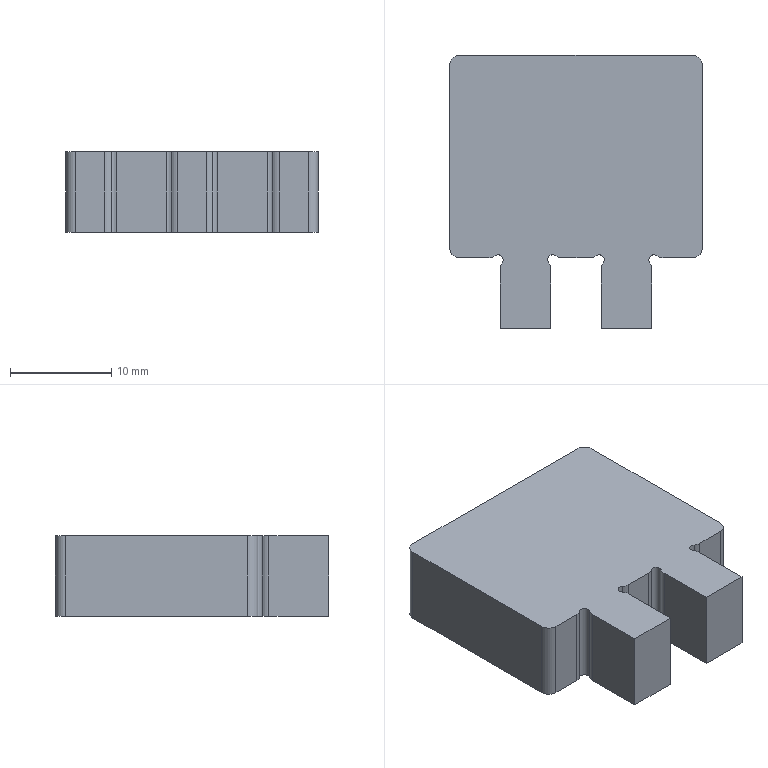Part | SolidWorks | features Fillet 1, FlatPattern 1, ICE 1, SMBaseFlange 1, SheetMetal 1 | 1 solid | 32 faces | box 25 x 27 x 8 mm | volume 4541 mm3 | cylinder 18 | plane 14 | commonest cylinder face diameters 2 x12 1 x6
STEP:
#1=CARTESIAN_POINT('',(52.732,-33.449,0.));
#2=VERTEX_POINT('',#1);
#3=CARTESIAN_POINT('',(51.932,-33.849,0.));
#4=VERTEX_POINT('',#3);
#5=CARTESIAN_POINT('',(52.432,-33.849,0.));
#6=DIRECTION('',(0.,0.,1.));
#7=DIRECTION('',(1.,0.,0.));
#8=AXIS2_PLACEMENT_3D('',#5,#6,#7);
#9=CIRCLE('',#8,0.5);
#10=EDGE_CURVE('',#2,#4,#9,.T.);
#11=ORIENTED_EDGE('',*,*,#10,.T.);
#12=CARTESIAN_POINT('',(51.932,-33.849,-8.));
#13=VERTEX_POINT('',#12);
#14=CARTESIAN_POINT('',(51.932,-33.849,-8.));
#15=DIRECTION('',(0.,0.,-1.));
#16=VECTOR('',#15,1000.);
#17=LINE('',#14,#16);
#18=EDGE_CURVE('',#4,#13,#17,.T.);
#19=ORIENTED_EDGE('',*,*,#18,.T.);
#20=CARTESIAN_POINT('',(52.732,-33.449,-8.));
#21=VERTEX_POINT('',#20);
#22=CARTESIAN_POINT('',(52.432,-33.849,-8.));
#23=DIRECTION('',(0.,0.,1.));
#24=DIRECTION('',(1.,0.,0.));
#25=AXIS2_PLACEMENT_3D('',#22,#23,#24);
#26=CIRCLE('',#25,0.5);
#27=EDGE_CURVE('',#21,#13,#26,.T.);
#28=ORIENTED_EDGE('',*,*,#27,.F.);
#29=CARTESIAN_POINT('',(52.732,-33.449,-8.));
#30=DIRECTION('',(0.,0.,1.));
#31=VECTOR('',#30,1000.);
#32=LINE('',#29,#31);
#33=EDGE_CURVE('',#21,#2,#32,.T.);
#34=ORIENTED_EDGE('',*,*,#33,.T.);
#35=EDGE_LOOP('',(#11,#19,#28,#34));
#36=FACE_OUTER_BOUND('',#35,.T.);
#37=CARTESIAN_POINT('',(52.432,-33.849,-8.));
#38=DIRECTION('',(0.,0.,-1.));
#39=DIRECTION('',(-1.,0.,0.));
#40=AXIS2_PLACEMENT_3D('',#37,#38,#39);
#41=CYLINDRICAL_SURFACE('',#40,0.5);
#42=ADVANCED_FACE('',(#36),#41,.F.);
#43=CARTESIAN_POINT('',(42.732,-33.449,0.));
#44=VERTEX_POINT('',#43);
#45=CARTESIAN_POINT('',(41.932,-33.849,0.));
#46=VERTEX_POINT('',#45);
#47=CARTESIAN_POINT('',(42.432,-33.849,0.));
#48=DIRECTION('',(0.,0.,1.));
#49=DIRECTION('',(1.,0.,0.));
#50=AXIS2_PLACEMENT_3D('',#47,#48,#49);
#51=CIRCLE('',#50,0.5);
#52=EDGE_CURVE('',#44,#46,#51,.T.);
#53=ORIENTED_EDGE('',*,*,#52,.T.);
#54=CARTESIAN_POINT('',(41.932,-33.849,-8.));
#55=VERTEX_POINT('',#54);
#56=CARTESIAN_POINT('',(41.932,-33.849,-8.));
#57=DIRECTION('',(0.,0.,-1.));
#58=VECTOR('',#57,1000.);
#59=LINE('',#56,#58);
#60=EDGE_CURVE('',#46,#55,#59,.T.);
#61=ORIENTED_EDGE('',*,*,#60,.T.);
#62=CARTESIAN_POINT('',(42.732,-33.449,-8.));
#63=VERTEX_POINT('',#62);
#64=CARTESIAN_POINT('',(42.432,-33.849,-8.));
#65=DIRECTION('',(0.,0.,1.));
#66=DIRECTION('',(1.,0.,0.));
#67=AXIS2_PLACEMENT_3D('',#64,#65,#66);
#68=CIRCLE('',#67,0.5);
#69=EDGE_CURVE('',#63,#55,#68,.T.);
#70=ORIENTED_EDGE('',*,*,#69,.F.);
#71=CARTESIAN_POINT('',(42.732,-33.449,-8.));
#72=DIRECTION('',(0.,0.,1.));
#73=VECTOR('',#72,1000.);
#74=LINE('',#71,#73);
#75=EDGE_CURVE('',#63,#44,#74,.T.);
#76=ORIENTED_EDGE('',*,*,#75,.T.);
#77=EDGE_LOOP('',(#53,#61,#70,#76));
#78=FACE_OUTER_BOUND('',#77,.T.);
#79=CARTESIAN_POINT('',(42.432,-33.849,-8.));
#80=DIRECTION('',(0.,0.,-1.));
#81=DIRECTION('',(-1.,0.,0.));
#82=AXIS2_PLACEMENT_3D('',#79,#80,#81);
#83=CYLINDRICAL_SURFACE('',#82,0.5);
#84=ADVANCED_FACE('',(#78),#83,.F.);
#85=CARTESIAN_POINT('',(33.232,-33.649,-8.));
#86=VERTEX_POINT('',#85);
#87=CARTESIAN_POINT('',(36.132,-33.649,-8.));
#88=VERTEX_POINT('',#87);
#89=CARTESIAN_POINT('',(37.232,-33.649,-8.));
#90=DIRECTION('',(1.,0.,0.));
#91=VECTOR('',#90,1000.);
#92=LINE('',#89,#91);
#93=EDGE_CURVE('',#86,#88,#92,.T.);
#94=ORIENTED_EDGE('',*,*,#93,.T.);
#95=CARTESIAN_POINT('',(36.132,-33.649,0.));
#96=VERTEX_POINT('',#95);
#97=CARTESIAN_POINT('',(36.132,-33.649,-8.));
#98=DIRECTION('',(0.,0.,1.));
#99=VECTOR('',#98,1000.);
#100=LINE('',#97,#99);
#101=EDGE_CURVE('',#88,#96,#100,.T.);
#102=ORIENTED_EDGE('',*,*,#101,.T.);
#103=CARTESIAN_POINT('',(33.232,-33.649,0.));
#104=VERTEX_POINT('',#103);
#105=CARTESIAN_POINT('',(37.232,-33.649,0.));
#106=DIRECTION('',(1.,0.,0.));
#107=VECTOR('',#106,1000.);
#108=LINE('',#105,#107);
#109=EDGE_CURVE('',#104,#96,#108,.T.);
#110=ORIENTED_EDGE('',*,*,#109,.F.);
#111=CARTESIAN_POINT('',(33.232,-33.649,-8.));
#112=DIRECTION('',(0.,0.,-1.));
#113=VECTOR('',#112,1000.);
#114=LINE('',#111,#113);
#115=EDGE_CURVE('',#104,#86,#114,.T.);
#116=ORIENTED_EDGE('',*,*,#115,.T.);
#117=EDGE_LOOP('',(#94,#102,#110,#116));
#118=FACE_OUTER_BOUND('',#117,.T.);
#119=CARTESIAN_POINT('',(37.232,-33.649,-8.));
#120=DIRECTION('',(0.,-1.,0.));
#121=DIRECTION('',(0.,0.,-1.));
#122=AXIS2_PLACEMENT_3D('',#119,#120,#121);
#123=PLANE('',#122);
#124=ADVANCED_FACE('',(#118),#123,.T.);
#125=CARTESIAN_POINT('',(53.332,-33.649,0.));
#126=VERTEX_POINT('',#125);
#127=CARTESIAN_POINT('',(56.232,-33.649,0.));
#128=VERTEX_POINT('',#127);
#129=CARTESIAN_POINT('',(57.232,-33.649,0.));
#130=DIRECTION('',(1.,0.,0.));
#131=VECTOR('',#130,1000.);
#132=LINE('',#129,#131);
#133=EDGE_CURVE('',#126,#128,#132,.T.);
#134=ORIENTED_EDGE('',*,*,#133,.F.);
#135=CARTESIAN_POINT('',(53.332,-33.649,-8.));
#136=VERTEX_POINT('',#135);
#137=CARTESIAN_POINT('',(53.332,-33.649,-8.));
#138=DIRECTION('',(0.,0.,-1.));
#139=VECTOR('',#138,1000.);
#140=LINE('',#137,#139);
#141=EDGE_CURVE('',#126,#136,#140,.T.);
#142=ORIENTED_EDGE('',*,*,#141,.T.);
#143=CARTESIAN_POINT('',(56.232,-33.649,-8.));
#144=VERTEX_POINT('',#143);
#145=CARTESIAN_POINT('',(57.232,-33.649,-8.));
#146=DIRECTION('',(1.,0.,0.));
#147=VECTOR('',#146,1000.);
#148=LINE('',#145,#147);
#149=EDGE_CURVE('',#136,#144,#148,.T.);
#150=ORIENTED_EDGE('',*,*,#149,.T.);
#151=CARTESIAN_POINT('',(56.232,-33.649,-8.));
#152=DIRECTION('',(0.,0.,1.));
#153=VECTOR('',#152,1000.);
#154=LINE('',#151,#153);
#155=EDGE_CURVE('',#144,#128,#154,.T.);
#156=ORIENTED_EDGE('',*,*,#155,.T.);
#157=EDGE_LOOP('',(#134,#142,#150,#156));
#158=FACE_OUTER_BOUND('',#157,.T.);
#159=CARTESIAN_POINT('',(57.232,-33.649,-8.));
#160=DIRECTION('',(0.,-1.,0.));
#161=DIRECTION('',(1.,0.,0.));
#162=AXIS2_PLACEMENT_3D('',#159,#160,#161);
#163=PLANE('',#162);
#164=ADVANCED_FACE('',(#158),#163,.T.);
#165=CARTESIAN_POINT('',(52.232,-40.649,-8.));
#166=VERTEX_POINT('',#165);
#167=CARTESIAN_POINT('',(52.232,-34.749,-8.));
#168=VERTEX_POINT('',#167);
#169=CARTESIAN_POINT('',(52.232,-33.649,-8.));
#170=DIRECTION('',(0.,1.,0.));
#171=VECTOR('',#170,1000.);
#172=LINE('',#169,#171);
#173=EDGE_CURVE('',#166,#168,#172,.T.);
#174=ORIENTED_EDGE('',*,*,#173,.T.);
#175=CARTESIAN_POINT('',(52.232,-34.749,0.));
#176=VERTEX_POINT('',#175);
#177=CARTESIAN_POINT('',(52.232,-34.749,-8.));
#178=DIRECTION('',(0.,0.,1.));
#179=VECTOR('',#178,1000.);
#180=LINE('',#177,#179);
#181=EDGE_CURVE('',#168,#176,#180,.T.);
#182=ORIENTED_EDGE('',*,*,#181,.T.);
#183=CARTESIAN_POINT('',(52.232,-40.649,0.));
#184=VERTEX_POINT('',#183);
#185=CARTESIAN_POINT('',(52.232,-33.649,0.));
#186=DIRECTION('',(0.,1.,0.));
#187=VECTOR('',#186,1000.);
#188=LINE('',#185,#187);
#189=EDGE_CURVE('',#184,#176,#188,.T.);
#190=ORIENTED_EDGE('',*,*,#189,.F.);
#191=CARTESIAN_POINT('',(52.232,-40.649,-8.));
#192=DIRECTION('',(0.,0.,1.));
#193=VECTOR('',#192,1000.);
#194=LINE('',#191,#193);
#195=EDGE_CURVE('',#166,#184,#194,.T.);
#196=ORIENTED_EDGE('',*,*,#195,.F.);
#197=EDGE_LOOP('',(#174,#182,#190,#196));
#198=FACE_OUTER_BOUND('',#197,.T.);
#199=CARTESIAN_POINT('',(52.232,-33.649,-8.));
#200=DIRECTION('',(1.,0.,0.));
#201=DIRECTION('',(0.,0.,-1.));
#202=AXIS2_PLACEMENT_3D('',#199,#200,#201);
#203=PLANE('',#202);
#204=ADVANCED_FACE('',(#198),#203,.T.);
#205=CARTESIAN_POINT('',(47.232,-34.749,0.));
#206=VERTEX_POINT('',#205);
#207=CARTESIAN_POINT('',(47.232,-40.649,0.));
#208=VERTEX_POINT('',#207);
#209=CARTESIAN_POINT('',(47.232,-40.649,0.));
#210=DIRECTION('',(0.,-1.,0.));
#211=VECTOR('',#210,1000.);
#212=LINE('',#209,#211);
#213=EDGE_CURVE('',#206,#208,#212,.T.);
#214=ORIENTED_EDGE('',*,*,#213,.F.);
#215=CARTESIAN_POINT('',(47.232,-34.749,-8.));
#216=VERTEX_POINT('',#215);
#217=CARTESIAN_POINT('',(47.232,-34.749,-8.));
#218=DIRECTION('',(0.,0.,-1.));
#219=VECTOR('',#218,1000.);
#220=LINE('',#217,#219);
#221=EDGE_CURVE('',#206,#216,#220,.T.);
#222=ORIENTED_EDGE('',*,*,#221,.T.);
#223=CARTESIAN_POINT('',(47.232,-40.649,-8.));
#224=VERTEX_POINT('',#223);
#225=CARTESIAN_POINT('',(47.232,-40.649,-8.));
#226=DIRECTION('',(0.,-1.,0.));
#227=VECTOR('',#226,1000.);
#228=LINE('',#225,#227);
#229=EDGE_CURVE('',#216,#224,#228,.T.);
#230=ORIENTED_EDGE('',*,*,#229,.T.);
#231=CARTESIAN_POINT('',(47.232,-40.649,-8.));
#232=DIRECTION('',(0.,0.,1.));
#233=VECTOR('',#232,1000.);
#234=LINE('',#231,#233);
#235=EDGE_CURVE('',#224,#208,#234,.T.);
#236=ORIENTED_EDGE('',*,*,#235,.T.);
#237=EDGE_LOOP('',(#214,#222,#230,#236));
#238=FACE_OUTER_BOUND('',#237,.T.);
#239=CARTESIAN_POINT('',(47.232,-40.649,-8.));
#240=DIRECTION('',(-1.,0.,0.));
#241=DIRECTION('',(0.,0.,1.));
#242=AXIS2_PLACEMENT_3D('',#239,#240,#241);
#243=PLANE('',#242);
#244=ADVANCED_FACE('',(#238),#243,.T.);
#245=CARTESIAN_POINT('',(43.332,-33.649,-8.));
#246=VERTEX_POINT('',#245);
#247=CARTESIAN_POINT('',(46.132,-33.649,-8.));
#248=VERTEX_POINT('',#247);
#249=CARTESIAN_POINT('',(47.232,-33.649,-8.));
#250=DIRECTION('',(1.,0.,0.));
#251=VECTOR('',#250,1000.);
#252=LINE('',#249,#251);
#253=EDGE_CURVE('',#246,#248,#252,.T.);
#254=ORIENTED_EDGE('',*,*,#253,.T.);
#255=CARTESIAN_POINT('',(46.132,-33.649,0.));
#256=VERTEX_POINT('',#255);
#257=CARTESIAN_POINT('',(46.132,-33.649,-8.));
#258=DIRECTION('',(0.,0.,1.));
#259=VECTOR('',#258,1000.);
#260=LINE('',#257,#259);
#261=EDGE_CURVE('',#248,#256,#260,.T.);
#262=ORIENTED_EDGE('',*,*,#261,.T.);
#263=CARTESIAN_POINT('',(43.332,-33.649,0.));
#264=VERTEX_POINT('',#263);
#265=CARTESIAN_POINT('',(47.232,-33.649,0.));
#266=DIRECTION('',(1.,0.,0.));
#267=VECTOR('',#266,1000.);
#268=LINE('',#265,#267);
#269=EDGE_CURVE('',#264,#256,#268,.T.);
#270=ORIENTED_EDGE('',*,*,#269,.F.);
#271=CARTESIAN_POINT('',(43.332,-33.649,-8.));
#272=DIRECTION('',(0.,0.,-1.));
#273=VECTOR('',#272,1000.);
#274=LINE('',#271,#273);
#275=EDGE_CURVE('',#264,#246,#274,.T.);
#276=ORIENTED_EDGE('',*,*,#275,.T.);
#277=EDGE_LOOP('',(#254,#262,#270,#276));
#278=FACE_OUTER_BOUND('',#277,.T.);
#279=CARTESIAN_POINT('',(47.232,-33.649,-8.));
#280=DIRECTION('',(0.,-1.,0.));
#281=DIRECTION('',(1.,0.,0.));
#282=AXIS2_PLACEMENT_3D('',#279,#280,#281);
#283=PLANE('',#282);
#284=ADVANCED_FACE('',(#278),#283,.T.);
#285=CARTESIAN_POINT('',(42.232,-40.649,-8.));
#286=VERTEX_POINT('',#285);
#287=CARTESIAN_POINT('',(42.232,-34.749,-8.));
#288=VERTEX_POINT('',#287);
#289=CARTESIAN_POINT('',(42.232,-33.649,-8.));
#290=DIRECTION('',(0.,1.,0.));
#291=VECTOR('',#290,1000.);
#292=LINE('',#289,#291);
#293=EDGE_CURVE('',#286,#288,#292,.T.);
#294=ORIENTED_EDGE('',*,*,#293,.T.);
#295=CARTESIAN_POINT('',(42.232,-34.749,0.));
#296=VERTEX_POINT('',#295);
#297=CARTESIAN_POINT('',(42.232,-34.749,-8.));
#298=DIRECTION('',(0.,0.,1.));
#299=VECTOR('',#298,1000.);
#300=LINE('',#297,#299);
#301=EDGE_CURVE('',#288,#296,#300,.T.);
#302=ORIENTED_EDGE('',*,*,#301,.T.);
#303=CARTESIAN_POINT('',(42.232,-40.649,0.));
#304=VERTEX_POINT('',#303);
#305=CARTESIAN_POINT('',(42.232,-33.649,0.));
#306=DIRECTION('',(0.,1.,0.));
#307=VECTOR('',#306,1000.);
#308=LINE('',#305,#307);
#309=EDGE_CURVE('',#304,#296,#308,.T.);
#310=ORIENTED_EDGE('',*,*,#309,.F.);
#311=CARTESIAN_POINT('',(42.232,-40.649,-8.));
#312=DIRECTION('',(0.,0.,1.));
#313=VECTOR('',#312,1000.);
#314=LINE('',#311,#313);
#315=EDGE_CURVE('',#286,#304,#314,.T.);
#316=ORIENTED_EDGE('',*,*,#315,.F.);
#317=EDGE_LOOP('',(#294,#302,#310,#316));
#318=FACE_OUTER_BOUND('',#317,.T.);
#319=CARTESIAN_POINT('',(42.232,-33.649,-8.));
#320=DIRECTION('',(1.,0.,0.));
#321=DIRECTION('',(0.,0.,-1.));
#322=AXIS2_PLACEMENT_3D('',#319,#320,#321);
#323=PLANE('',#322);
#324=ADVANCED_FACE('',(#318),#323,.T.);
#325=CARTESIAN_POINT('',(37.232,-34.749,0.));
#326=VERTEX_POINT('',#325);
#327=CARTESIAN_POINT('',(37.232,-40.649,0.));
#328=VERTEX_POINT('',#327);
#329=CARTESIAN_POINT('',(37.232,-40.649,0.));
#330=DIRECTION('',(0.,-1.,0.));
#331=VECTOR('',#330,1000.);
#332=LINE('',#329,#331);
#333=EDGE_CURVE('',#326,#328,#332,.T.);
#334=ORIENTED_EDGE('',*,*,#333,.F.);
#335=CARTESIAN_POINT('',(37.232,-34.749,-8.));
#336=VERTEX_POINT('',#335);
#337=CARTESIAN_POINT('',(37.232,-34.749,-8.));
#338=DIRECTION('',(0.,0.,-1.));
#339=VECTOR('',#338,1000.);
#340=LINE('',#337,#339);
#341=EDGE_CURVE('',#326,#336,#340,.T.);
#342=ORIENTED_EDGE('',*,*,#341,.T.);
#343=CARTESIAN_POINT('',(37.232,-40.649,-8.));
#344=VERTEX_POINT('',#343);
#345=CARTESIAN_POINT('',(37.232,-40.649,-8.));
#346=DIRECTION('',(0.,-1.,0.));
#347=VECTOR('',#346,1000.);
#348=LINE('',#345,#347);
#349=EDGE_CURVE('',#336,#344,#348,.T.);
#350=ORIENTED_EDGE('',*,*,#349,.T.);
#351=CARTESIAN_POINT('',(37.232,-40.649,-8.));
#352=DIRECTION('',(0.,0.,1.));
#353=VECTOR('',#352,1000.);
#354=LINE('',#351,#353);
#355=EDGE_CURVE('',#344,#328,#354,.T.);
#356=ORIENTED_EDGE('',*,*,#355,.T.);
#357=EDGE_LOOP('',(#334,#342,#350,#356));
#358=FACE_OUTER_BOUND('',#357,.T.);
#359=CARTESIAN_POINT('',(37.232,-40.649,-8.));
#360=DIRECTION('',(-1.,0.,0.));
#361=DIRECTION('',(0.,0.,1.));
#362=AXIS2_PLACEMENT_3D('',#359,#360,#361);
#363=PLANE('',#362);
#364=ADVANCED_FACE('',(#358),#363,.T.);
#365=CARTESIAN_POINT('',(32.232,-14.649,-8.));
#366=VERTEX_POINT('',#365);
#367=CARTESIAN_POINT('',(32.232,-32.649,-8.));
#368=VERTEX_POINT('',#367);
#369=CARTESIAN_POINT('',(32.232,-33.649,-8.));
#370=DIRECTION('',(0.,-1.,0.));
#371=VECTOR('',#370,1000.);
#372=LINE('',#369,#371);
#373=EDGE_CURVE('',#366,#368,#372,.T.);
#374=ORIENTED_EDGE('',*,*,#373,.T.);
#375=CARTESIAN_POINT('',(32.232,-32.649,0.));
#376=VERTEX_POINT('',#375);
#377=CARTESIAN_POINT('',(32.232,-32.649,-8.));
#378=DIRECTION('',(0.,0.,1.));
#379=VECTOR('',#378,1000.);
#380=LINE('',#377,#379);
#381=EDGE_CURVE('',#368,#376,#380,.T.);
#382=ORIENTED_EDGE('',*,*,#381,.T.);
#383=CARTESIAN_POINT('',(32.232,-14.649,0.));
#384=VERTEX_POINT('',#383);
#385=CARTESIAN_POINT('',(32.232,-33.649,0.));
#386=DIRECTION('',(0.,-1.,0.));
#387=VECTOR('',#386,1000.);
#388=LINE('',#385,#387);
#389=EDGE_CURVE('',#384,#376,#388,.T.);
#390=ORIENTED_EDGE('',*,*,#389,.F.);
#391=CARTESIAN_POINT('',(32.232,-14.649,-8.));
#392=DIRECTION('',(0.,0.,-1.));
#393=VECTOR('',#392,1000.);
#394=LINE('',#391,#393);
#395=EDGE_CURVE('',#384,#366,#394,.T.);
#396=ORIENTED_EDGE('',*,*,#395,.T.);
#397=EDGE_LOOP('',(#374,#382,#390,#396));
#398=FACE_OUTER_BOUND('',#397,.T.);
#399=CARTESIAN_POINT('',(32.232,-33.649,-8.));
#400=DIRECTION('',(-1.,0.,0.));
#401=DIRECTION('',(0.,0.,1.));
#402=AXIS2_PLACEMENT_3D('',#399,#400,#401);
#403=PLANE('',#402);
#404=ADVANCED_FACE('',(#398),#403,.T.);
#405=CARTESIAN_POINT('',(56.232,-13.649,-8.));
#406=VERTEX_POINT('',#405);
#407=CARTESIAN_POINT('',(33.232,-13.649,-8.));
#408=VERTEX_POINT('',#407);
#409=CARTESIAN_POINT('',(32.232,-13.649,-8.));
#410=DIRECTION('',(-1.,0.,0.));
#411=VECTOR('',#410,1000.);
#412=LINE('',#409,#411);
#413=EDGE_CURVE('',#406,#408,#412,.T.);
#414=ORIENTED_EDGE('',*,*,#413,.T.);
#415=CARTESIAN_POINT('',(33.232,-13.649,0.));
#416=VERTEX_POINT('',#415);
#417=CARTESIAN_POINT('',(33.232,-13.649,-8.));
#418=DIRECTION('',(0.,0.,1.));
#419=VECTOR('',#418,1000.);
#420=LINE('',#417,#419);
#421=EDGE_CURVE('',#408,#416,#420,.T.);
#422=ORIENTED_EDGE('',*,*,#421,.T.);
#423=CARTESIAN_POINT('',(56.232,-13.649,0.));
#424=VERTEX_POINT('',#423);
#425=CARTESIAN_POINT('',(32.232,-13.649,0.));
#426=DIRECTION('',(-1.,0.,0.));
#427=VECTOR('',#426,1000.);
#428=LINE('',#425,#427);
#429=EDGE_CURVE('',#424,#416,#428,.T.);
#430=ORIENTED_EDGE('',*,*,#429,.F.);
#431=CARTESIAN_POINT('',(56.232,-13.649,-8.));
#432=DIRECTION('',(0.,0.,-1.));
#433=VECTOR('',#432,1000.);
#434=LINE('',#431,#433);
#435=EDGE_CURVE('',#424,#406,#434,.T.);
#436=ORIENTED_EDGE('',*,*,#435,.T.);
#437=EDGE_LOOP('',(#414,#422,#430,#436));
#438=FACE_OUTER_BOUND('',#437,.T.);
#439=CARTESIAN_POINT('',(32.232,-13.649,-8.));
#440=DIRECTION('',(0.,1.,0.));
#441=DIRECTION('',(0.,0.,1.));
#442=AXIS2_PLACEMENT_3D('',#439,#440,#441);
#443=PLANE('',#442);
#444=ADVANCED_FACE('',(#438),#443,.T.);
#445=CARTESIAN_POINT('',(57.232,-32.649,0.));
#446=VERTEX_POINT('',#445);
#447=CARTESIAN_POINT('',(57.232,-14.649,0.));
#448=VERTEX_POINT('',#447);
#449=CARTESIAN_POINT('',(57.232,-13.649,0.));
#450=DIRECTION('',(0.,1.,0.));
#451=VECTOR('',#450,1000.);
#452=LINE('',#449,#451);
#453=EDGE_CURVE('',#446,#448,#452,.T.);
#454=ORIENTED_EDGE('',*,*,#453,.F.);
#455=CARTESIAN_POINT('',(57.232,-32.649,-8.));
#456=VERTEX_POINT('',#455);
#457=CARTESIAN_POINT('',(57.232,-32.649,-8.));
#458=DIRECTION('',(0.,0.,-1.));
#459=VECTOR('',#458,1000.);
#460=LINE('',#457,#459);
#461=EDGE_CURVE('',#446,#456,#460,.T.);
#462=ORIENTED_EDGE('',*,*,#461,.T.);
#463=CARTESIAN_POINT('',(57.232,-14.649,-8.));
#464=VERTEX_POINT('',#463);
#465=CARTESIAN_POINT('',(57.232,-13.649,-8.));
#466=DIRECTION('',(0.,1.,0.));
#467=VECTOR('',#466,1000.);
#468=LINE('',#465,#467);
#469=EDGE_CURVE('',#456,#464,#468,.T.);
#470=ORIENTED_EDGE('',*,*,#469,.T.);
#471=CARTESIAN_POINT('',(57.232,-14.649,-8.));
#472=DIRECTION('',(0.,0.,1.));
#473=VECTOR('',#472,1000.);
#474=LINE('',#471,#473);
#475=EDGE_CURVE('',#464,#448,#474,.T.);
#476=ORIENTED_EDGE('',*,*,#475,.T.);
#477=EDGE_LOOP('',(#454,#462,#470,#476));
#478=FACE_OUTER_BOUND('',#477,.T.);
#479=CARTESIAN_POINT('',(57.232,-13.649,-8.));
#480=DIRECTION('',(1.,0.,0.));
#481=DIRECTION('',(0.,0.,-1.));
#482=AXIS2_PLACEMENT_3D('',#479,#480,#481);
#483=PLANE('',#482);
#484=ADVANCED_FACE('',(#478),#483,.T.);
#485=CARTESIAN_POINT('',(52.232,-40.649,0.));
#486=DIRECTION('',(1.,0.,0.));
#487=VECTOR('',#486,1000.);
#488=LINE('',#485,#487);
#489=EDGE_CURVE('',#208,#184,#488,.T.);
#490=ORIENTED_EDGE('',*,*,#489,.F.);
#491=ORIENTED_EDGE('',*,*,#235,.F.);
#492=CARTESIAN_POINT('',(52.232,-40.649,-8.));
#493=DIRECTION('',(1.,0.,0.));
#494=VECTOR('',#493,1000.);
#495=LINE('',#492,#494);
#496=EDGE_CURVE('',#224,#166,#495,.T.);
#497=ORIENTED_EDGE('',*,*,#496,.T.);
#498=ORIENTED_EDGE('',*,*,#195,.T.);
#499=EDGE_LOOP('',(#490,#491,#497,#498));
#500=FACE_OUTER_BOUND('',#499,.T.);
#501=CARTESIAN_POINT('',(52.232,-40.649,-8.));
#502=DIRECTION('',(0.,-1.,0.));
#503=DIRECTION('',(1.,0.,0.));
#504=AXIS2_PLACEMENT_3D('',#501,#502,#503);
#505=PLANE('',#504);
#506=ADVANCED_FACE('',(#500),#505,.T.);
#507=CARTESIAN_POINT('',(42.232,-40.649,0.));
#508=DIRECTION('',(1.,0.,0.));
#509=VECTOR('',#508,1000.);
#510=LINE('',#507,#509);
#511=EDGE_CURVE('',#328,#304,#510,.T.);
#512=ORIENTED_EDGE('',*,*,#511,.F.);
#513=ORIENTED_EDGE('',*,*,#355,.F.);
#514=CARTESIAN_POINT('',(42.232,-40.649,-8.));
#515=DIRECTION('',(1.,0.,0.));
#516=VECTOR('',#515,1000.);
#517=LINE('',#514,#516);
#518=EDGE_CURVE('',#344,#286,#517,.T.);
#519=ORIENTED_EDGE('',*,*,#518,.T.);
#520=ORIENTED_EDGE('',*,*,#315,.T.);
#521=EDGE_LOOP('',(#512,#513,#519,#520));
#522=FACE_OUTER_BOUND('',#521,.T.);
#523=CARTESIAN_POINT('',(42.232,-40.649,-8.));
#524=DIRECTION('',(0.,-1.,0.));
#525=DIRECTION('',(0.,0.,-1.));
#526=AXIS2_PLACEMENT_3D('',#523,#524,#525);
#527=PLANE('',#526);
#528=ADVANCED_FACE('',(#522),#527,.T.);
#529=ORIENTED_EDGE('',*,*,#149,.F.);
#530=CARTESIAN_POINT('',(53.332,-32.649,-8.));
#531=DIRECTION('',(0.,0.,-1.));
#532=DIRECTION('',(-1.,0.,0.));
#533=AXIS2_PLACEMENT_3D('',#530,#531,#532);
#534=CIRCLE('',#533,1.);
#535=EDGE_CURVE('',#136,#21,#534,.T.);
#536=ORIENTED_EDGE('',*,*,#535,.T.);
#537=ORIENTED_EDGE('',*,*,#27,.T.);
#538=CARTESIAN_POINT('',(52.032,-34.149,-8.));
#539=VERTEX_POINT('',#538);
#540=CARTESIAN_POINT('',(52.432,-33.849,-8.));
#541=DIRECTION('',(0.,0.,1.));
#542=DIRECTION('',(1.,0.,0.));
#543=AXIS2_PLACEMENT_3D('',#540,#541,#542);
#544=CIRCLE('',#543,0.5);
#545=EDGE_CURVE('',#13,#539,#544,.T.);
#546=ORIENTED_EDGE('',*,*,#545,.T.);
#547=CARTESIAN_POINT('',(51.232,-34.749,-8.));
#548=DIRECTION('',(0.,0.,-1.));
#549=DIRECTION('',(-1.,0.,0.));
#550=AXIS2_PLACEMENT_3D('',#547,#548,#549);
#551=CIRCLE('',#550,1.);
#552=EDGE_CURVE('',#539,#168,#551,.T.);
#553=ORIENTED_EDGE('',*,*,#552,.T.);
#554=ORIENTED_EDGE('',*,*,#173,.F.);
#555=ORIENTED_EDGE('',*,*,#496,.F.);
#556=ORIENTED_EDGE('',*,*,#229,.F.);
#557=CARTESIAN_POINT('',(47.432,-34.149,-8.));
#558=VERTEX_POINT('',#557);
#559=CARTESIAN_POINT('',(48.232,-34.749,-8.));
#560=DIRECTION('',(0.,0.,-1.));
#561=DIRECTION('',(-1.,0.,0.));
#562=AXIS2_PLACEMENT_3D('',#559,#560,#561);
#563=CIRCLE('',#562,1.);
#564=EDGE_CURVE('',#216,#558,#563,.T.);
#565=ORIENTED_EDGE('',*,*,#564,.T.);
#566=CARTESIAN_POINT('',(46.732,-33.449,-8.));
#567=VERTEX_POINT('',#566);
#568=CARTESIAN_POINT('',(47.032,-33.849,-8.));
#569=DIRECTION('',(0.,0.,1.));
#570=DIRECTION('',(1.,0.,0.));
#571=AXIS2_PLACEMENT_3D('',#568,#569,#570);
#572=CIRCLE('',#571,0.5);
#573=EDGE_CURVE('',#558,#567,#572,.T.);
#574=ORIENTED_EDGE('',*,*,#573,.T.);
#575=CARTESIAN_POINT('',(46.132,-32.649,-8.));
#576=DIRECTION('',(0.,0.,-1.));
#577=DIRECTION('',(-1.,0.,0.));
#578=AXIS2_PLACEMENT_3D('',#575,#576,#577);
#579=CIRCLE('',#578,1.);
#580=EDGE_CURVE('',#567,#248,#579,.T.);
#581=ORIENTED_EDGE('',*,*,#580,.T.);
#582=ORIENTED_EDGE('',*,*,#253,.F.);
#583=CARTESIAN_POINT('',(43.332,-32.649,-8.));
#584=DIRECTION('',(0.,0.,-1.));
#585=DIRECTION('',(-1.,0.,0.));
#586=AXIS2_PLACEMENT_3D('',#583,#584,#585);
#587=CIRCLE('',#586,1.);
#588=EDGE_CURVE('',#246,#63,#587,.T.);
#589=ORIENTED_EDGE('',*,*,#588,.T.);
#590=ORIENTED_EDGE('',*,*,#69,.T.);
#591=CARTESIAN_POINT('',(42.032,-34.149,-8.));
#592=VERTEX_POINT('',#591);
#593=CARTESIAN_POINT('',(42.432,-33.849,-8.));
#594=DIRECTION('',(0.,0.,1.));
#595=DIRECTION('',(1.,0.,0.));
#596=AXIS2_PLACEMENT_3D('',#593,#594,#595);
#597=CIRCLE('',#596,0.5);
#598=EDGE_CURVE('',#55,#592,#597,.T.);
#599=ORIENTED_EDGE('',*,*,#598,.T.);
#600=CARTESIAN_POINT('',(41.232,-34.749,-8.));
#601=DIRECTION('',(0.,0.,-1.));
#602=DIRECTION('',(-1.,0.,0.));
#603=AXIS2_PLACEMENT_3D('',#600,#601,#602);
#604=CIRCLE('',#603,1.);
#605=EDGE_CURVE('',#592,#288,#604,.T.);
#606=ORIENTED_EDGE('',*,*,#605,.T.);
#607=ORIENTED_EDGE('',*,*,#293,.F.);
#608=ORIENTED_EDGE('',*,*,#518,.F.);
#609=ORIENTED_EDGE('',*,*,#349,.F.);
#610=CARTESIAN_POINT('',(37.432,-34.149,-8.));
#611=VERTEX_POINT('',#610);
#612=CARTESIAN_POINT('',(38.232,-34.749,-8.));
#613=DIRECTION('',(0.,0.,-1.));
#614=DIRECTION('',(-1.,0.,0.));
#615=AXIS2_PLACEMENT_3D('',#612,#613,#614);
#616=CIRCLE('',#615,1.);
#617=EDGE_CURVE('',#336,#611,#616,.T.);
#618=ORIENTED_EDGE('',*,*,#617,.T.);
#619=CARTESIAN_POINT('',(36.732,-33.449,-8.));
#620=VERTEX_POINT('',#619);
#621=CARTESIAN_POINT('',(37.032,-33.849,-8.));
#622=DIRECTION('',(0.,0.,-1.));
#623=DIRECTION('',(-1.,0.,0.));
#624=AXIS2_PLACEMENT_3D('',#621,#622,#623);
#625=CIRCLE('',#624,0.5);
#626=EDGE_CURVE('',#620,#611,#625,.T.);
#627=ORIENTED_EDGE('',*,*,#626,.F.);
#628=CARTESIAN_POINT('',(36.132,-32.649,-8.));
#629=DIRECTION('',(0.,0.,-1.));
#630=DIRECTION('',(-1.,0.,0.));
#631=AXIS2_PLACEMENT_3D('',#628,#629,#630);
#632=CIRCLE('',#631,1.);
#633=EDGE_CURVE('',#620,#88,#632,.T.);
#634=ORIENTED_EDGE('',*,*,#633,.T.);
#635=ORIENTED_EDGE('',*,*,#93,.F.);
#636=CARTESIAN_POINT('',(33.232,-32.649,-8.));
#637=DIRECTION('',(0.,0.,-1.));
#638=DIRECTION('',(-1.,0.,0.));
#639=AXIS2_PLACEMENT_3D('',#636,#637,#638);
#640=CIRCLE('',#639,1.);
#641=EDGE_CURVE('',#86,#368,#640,.T.);
#642=ORIENTED_EDGE('',*,*,#641,.T.);
#643=ORIENTED_EDGE('',*,*,#373,.F.);
#644=CARTESIAN_POINT('',(33.232,-14.649,-8.));
#645=DIRECTION('',(0.,0.,-1.));
#646=DIRECTION('',(-1.,0.,0.));
#647=AXIS2_PLACEMENT_3D('',#644,#645,#646);
#648=CIRCLE('',#647,1.);
#649=EDGE_CURVE('',#366,#408,#648,.T.);
#650=ORIENTED_EDGE('',*,*,#649,.T.);
#651=ORIENTED_EDGE('',*,*,#413,.F.);
#652=CARTESIAN_POINT('',(56.232,-14.649,-8.));
#653=DIRECTION('',(0.,0.,-1.));
#654=DIRECTION('',(-1.,0.,0.));
#655=AXIS2_PLACEMENT_3D('',#652,#653,#654);
#656=CIRCLE('',#655,1.);
#657=EDGE_CURVE('',#406,#464,#656,.T.);
#658=ORIENTED_EDGE('',*,*,#657,.T.);
#659=ORIENTED_EDGE('',*,*,#469,.F.);
#660=CARTESIAN_POINT('',(56.232,-32.649,-8.));
#661=DIRECTION('',(0.,0.,-1.));
#662=DIRECTION('',(-1.,0.,0.));
#663=AXIS2_PLACEMENT_3D('',#660,#661,#662);
#664=CIRCLE('',#663,1.);
#665=EDGE_CURVE('',#456,#144,#664,.T.);
#666=ORIENTED_EDGE('',*,*,#665,.T.);
#667=EDGE_LOOP('',(#529,#536,#537,#546,#553,#554,#555,#556,#565,#574,#581,#582,#589,#590,#599,#606,#607,#608,#609,#618,#627,#634,#635,#642,#643,#650,#651,#658,#659,#666));
#668=FACE_OUTER_BOUND('',#667,.T.);
#669=CARTESIAN_POINT('',(0.,0.,-8.));
#670=DIRECTION('',(0.,0.,-1.));
#671=DIRECTION('',(-1.,0.,0.));
#672=AXIS2_PLACEMENT_3D('',#669,#670,#671);
#673=PLANE('',#672);
#674=ADVANCED_FACE('',(#668),#673,.T.);
#675=ORIENTED_EDGE('',*,*,#10,.F.);
#676=CARTESIAN_POINT('',(53.332,-32.649,0.));
#677=DIRECTION('',(0.,0.,1.));
#678=DIRECTION('',(-1.,0.,0.));
#679=AXIS2_PLACEMENT_3D('',#676,#677,#678);
#680=CIRCLE('',#679,1.);
#681=EDGE_CURVE('',#2,#126,#680,.T.);
#682=ORIENTED_EDGE('',*,*,#681,.T.);
#683=ORIENTED_EDGE('',*,*,#133,.T.);
#684=CARTESIAN_POINT('',(56.232,-32.649,0.));
#685=DIRECTION('',(0.,0.,1.));
#686=DIRECTION('',(-1.,0.,0.));
#687=AXIS2_PLACEMENT_3D('',#684,#685,#686);
#688=CIRCLE('',#687,1.);
#689=EDGE_CURVE('',#128,#446,#688,.T.);
#690=ORIENTED_EDGE('',*,*,#689,.T.);
#691=ORIENTED_EDGE('',*,*,#453,.T.);
#692=CARTESIAN_POINT('',(56.232,-14.649,0.));
#693=DIRECTION('',(0.,0.,1.));
#694=DIRECTION('',(-1.,0.,0.));
#695=AXIS2_PLACEMENT_3D('',#692,#693,#694);
#696=CIRCLE('',#695,1.);
#697=EDGE_CURVE('',#448,#424,#696,.T.);
#698=ORIENTED_EDGE('',*,*,#697,.T.);
#699=ORIENTED_EDGE('',*,*,#429,.T.);
#700=CARTESIAN_POINT('',(33.232,-14.649,0.));
#701=DIRECTION('',(0.,0.,1.));
#702=DIRECTION('',(-1.,0.,0.));
#703=AXIS2_PLACEMENT_3D('',#700,#701,#702);
#704=CIRCLE('',#703,1.);
#705=EDGE_CURVE('',#416,#384,#704,.T.);
#706=ORIENTED_EDGE('',*,*,#705,.T.);
#707=ORIENTED_EDGE('',*,*,#389,.T.);
#708=CARTESIAN_POINT('',(33.232,-32.649,0.));
#709=DIRECTION('',(0.,0.,1.));
#710=DIRECTION('',(-1.,0.,0.));
#711=AXIS2_PLACEMENT_3D('',#708,#709,#710);
#712=CIRCLE('',#711,1.);
#713=EDGE_CURVE('',#376,#104,#712,.T.);
#714=ORIENTED_EDGE('',*,*,#713,.T.);
#715=ORIENTED_EDGE('',*,*,#109,.T.);
#716=CARTESIAN_POINT('',(36.732,-33.449,0.));
#717=VERTEX_POINT('',#716);
#718=CARTESIAN_POINT('',(36.132,-32.649,0.));
#719=DIRECTION('',(0.,0.,1.));
#720=DIRECTION('',(-1.,0.,0.));
#721=AXIS2_PLACEMENT_3D('',#718,#719,#720);
#722=CIRCLE('',#721,1.);
#723=EDGE_CURVE('',#96,#717,#722,.T.);
#724=ORIENTED_EDGE('',*,*,#723,.T.);
#725=CARTESIAN_POINT('',(37.432,-34.149,0.));
#726=VERTEX_POINT('',#725);
#727=CARTESIAN_POINT('',(37.032,-33.849,0.));
#728=DIRECTION('',(0.,0.,-1.));
#729=DIRECTION('',(-1.,0.,0.));
#730=AXIS2_PLACEMENT_3D('',#727,#728,#729);
#731=CIRCLE('',#730,0.5);
#732=EDGE_CURVE('',#717,#726,#731,.T.);
#733=ORIENTED_EDGE('',*,*,#732,.T.);
#734=CARTESIAN_POINT('',(38.232,-34.749,0.));
#735=DIRECTION('',(0.,0.,1.));
#736=DIRECTION('',(-1.,0.,0.));
#737=AXIS2_PLACEMENT_3D('',#734,#735,#736);
#738=CIRCLE('',#737,1.);
#739=EDGE_CURVE('',#726,#326,#738,.T.);
#740=ORIENTED_EDGE('',*,*,#739,.T.);
#741=ORIENTED_EDGE('',*,*,#333,.T.);
#742=ORIENTED_EDGE('',*,*,#511,.T.);
#743=ORIENTED_EDGE('',*,*,#309,.T.);
#744=CARTESIAN_POINT('',(42.032,-34.149,0.));
#745=VERTEX_POINT('',#744);
#746=CARTESIAN_POINT('',(41.232,-34.749,0.));
#747=DIRECTION('',(0.,0.,1.));
#748=DIRECTION('',(-1.,0.,0.));
#749=AXIS2_PLACEMENT_3D('',#746,#747,#748);
#750=CIRCLE('',#749,1.);
#751=EDGE_CURVE('',#296,#745,#750,.T.);
#752=ORIENTED_EDGE('',*,*,#751,.T.);
#753=CARTESIAN_POINT('',(42.432,-33.849,0.));
#754=DIRECTION('',(0.,0.,1.));
#755=DIRECTION('',(1.,0.,0.));
#756=AXIS2_PLACEMENT_3D('',#753,#754,#755);
#757=CIRCLE('',#756,0.5);
#758=EDGE_CURVE('',#46,#745,#757,.T.);
#759=ORIENTED_EDGE('',*,*,#758,.F.);
#760=ORIENTED_EDGE('',*,*,#52,.F.);
#761=CARTESIAN_POINT('',(43.332,-32.649,0.));
#762=DIRECTION('',(0.,0.,1.));
#763=DIRECTION('',(-1.,0.,0.));
#764=AXIS2_PLACEMENT_3D('',#761,#762,#763);
#765=CIRCLE('',#764,1.);
#766=EDGE_CURVE('',#44,#264,#765,.T.);
#767=ORIENTED_EDGE('',*,*,#766,.T.);
#768=ORIENTED_EDGE('',*,*,#269,.T.);
#769=CARTESIAN_POINT('',(46.732,-33.449,0.));
#770=VERTEX_POINT('',#769);
#771=CARTESIAN_POINT('',(46.132,-32.649,0.));
#772=DIRECTION('',(0.,0.,1.));
#773=DIRECTION('',(-1.,0.,0.));
#774=AXIS2_PLACEMENT_3D('',#771,#772,#773);
#775=CIRCLE('',#774,1.);
#776=EDGE_CURVE('',#256,#770,#775,.T.);
#777=ORIENTED_EDGE('',*,*,#776,.T.);
#778=CARTESIAN_POINT('',(47.432,-34.149,0.));
#779=VERTEX_POINT('',#778);
#780=CARTESIAN_POINT('',(47.032,-33.849,0.));
#781=DIRECTION('',(0.,0.,1.));
#782=DIRECTION('',(1.,0.,0.));
#783=AXIS2_PLACEMENT_3D('',#780,#781,#782);
#784=CIRCLE('',#783,0.5);
#785=EDGE_CURVE('',#779,#770,#784,.T.);
#786=ORIENTED_EDGE('',*,*,#785,.F.);
#787=CARTESIAN_POINT('',(48.232,-34.749,0.));
#788=DIRECTION('',(0.,0.,1.));
#789=DIRECTION('',(-1.,0.,0.));
#790=AXIS2_PLACEMENT_3D('',#787,#788,#789);
#791=CIRCLE('',#790,1.);
#792=EDGE_CURVE('',#779,#206,#791,.T.);
#793=ORIENTED_EDGE('',*,*,#792,.T.);
#794=ORIENTED_EDGE('',*,*,#213,.T.);
#795=ORIENTED_EDGE('',*,*,#489,.T.);
#796=ORIENTED_EDGE('',*,*,#189,.T.);
#797=CARTESIAN_POINT('',(52.032,-34.149,0.));
#798=VERTEX_POINT('',#797);
#799=CARTESIAN_POINT('',(51.232,-34.749,0.));
#800=DIRECTION('',(0.,0.,1.));
#801=DIRECTION('',(-1.,0.,0.));
#802=AXIS2_PLACEMENT_3D('',#799,#800,#801);
#803=CIRCLE('',#802,1.);
#804=EDGE_CURVE('',#176,#798,#803,.T.);
#805=ORIENTED_EDGE('',*,*,#804,.T.);
#806=CARTESIAN_POINT('',(52.432,-33.849,0.));
#807=DIRECTION('',(0.,0.,1.));
#808=DIRECTION('',(1.,0.,0.));
#809=AXIS2_PLACEMENT_3D('',#806,#807,#808);
#810=CIRCLE('',#809,0.5);
#811=EDGE_CURVE('',#4,#798,#810,.T.);
#812=ORIENTED_EDGE('',*,*,#811,.F.);
#813=EDGE_LOOP('',(#675,#682,#683,#690,#691,#698,#699,#706,#707,#714,#715,#724,#733,#740,#741,#742,#743,#752,#759,#760,#767,#768,#777,#786,#793,#794,#795,#796,#805,#812));
#814=FACE_OUTER_BOUND('',#813,.T.);
#815=CARTESIAN_POINT('',(0.,0.,0.));
#816=DIRECTION('',(0.,0.,-1.));
#817=DIRECTION('',(-1.,0.,0.));
#818=AXIS2_PLACEMENT_3D('',#815,#816,#817);
#819=PLANE('',#818);
#820=ADVANCED_FACE('',(#814),#819,.F.);
#821=ORIENTED_EDGE('',*,*,#573,.F.);
#822=CARTESIAN_POINT('',(47.432,-34.149,-8.));
#823=DIRECTION('',(0.,0.,1.));
#824=VECTOR('',#823,1000.);
#825=LINE('',#822,#824);
#826=EDGE_CURVE('',#558,#779,#825,.T.);
#827=ORIENTED_EDGE('',*,*,#826,.T.);
#828=ORIENTED_EDGE('',*,*,#785,.T.);
#829=CARTESIAN_POINT('',(46.732,-33.449,-8.));
#830=DIRECTION('',(0.,0.,-1.));
#831=VECTOR('',#830,1000.);
#832=LINE('',#829,#831);
#833=EDGE_CURVE('',#770,#567,#832,.T.);
#834=ORIENTED_EDGE('',*,*,#833,.T.);
#835=EDGE_LOOP('',(#821,#827,#828,#834));
#836=FACE_OUTER_BOUND('',#835,.T.);
#837=CARTESIAN_POINT('',(47.032,-33.849,-8.));
#838=DIRECTION('',(0.,0.,-1.));
#839=DIRECTION('',(-1.,0.,0.));
#840=AXIS2_PLACEMENT_3D('',#837,#838,#839);
#841=CYLINDRICAL_SURFACE('',#840,0.5);
#842=ADVANCED_FACE('',(#836),#841,.F.);
#843=ORIENTED_EDGE('',*,*,#60,.F.);
#844=ORIENTED_EDGE('',*,*,#758,.T.);
#845=CARTESIAN_POINT('',(42.032,-34.149,-8.));
#846=DIRECTION('',(0.,0.,-1.));
#847=VECTOR('',#846,1000.);
#848=LINE('',#845,#847);
#849=EDGE_CURVE('',#745,#592,#848,.T.);
#850=ORIENTED_EDGE('',*,*,#849,.T.);
#851=ORIENTED_EDGE('',*,*,#598,.F.);
#852=EDGE_LOOP('',(#843,#844,#850,#851));
#853=FACE_OUTER_BOUND('',#852,.T.);
#854=CARTESIAN_POINT('',(42.432,-33.849,-8.));
#855=DIRECTION('',(0.,0.,-1.));
#856=DIRECTION('',(-1.,0.,0.));
#857=AXIS2_PLACEMENT_3D('',#854,#855,#856);
#858=CYLINDRICAL_SURFACE('',#857,0.5);
#859=ADVANCED_FACE('',(#853),#858,.F.);
#860=ORIENTED_EDGE('',*,*,#626,.T.);
#861=CARTESIAN_POINT('',(37.432,-34.149,0.));
#862=DIRECTION('',(0.,0.,1.));
#863=VECTOR('',#862,1000.);
#864=LINE('',#861,#863);
#865=EDGE_CURVE('',#611,#726,#864,.T.);
#866=ORIENTED_EDGE('',*,*,#865,.T.);
#867=ORIENTED_EDGE('',*,*,#732,.F.);
#868=CARTESIAN_POINT('',(36.732,-33.449,0.));
#869=DIRECTION('',(0.,0.,-1.));
#870=VECTOR('',#869,1000.);
#871=LINE('',#868,#870);
#872=EDGE_CURVE('',#717,#620,#871,.T.);
#873=ORIENTED_EDGE('',*,*,#872,.T.);
#874=EDGE_LOOP('',(#860,#866,#867,#873));
#875=FACE_OUTER_BOUND('',#874,.T.);
#876=CARTESIAN_POINT('',(37.032,-33.849,0.));
#877=DIRECTION('',(0.,0.,-1.));
#878=DIRECTION('',(-1.,0.,0.));
#879=AXIS2_PLACEMENT_3D('',#876,#877,#878);
#880=CYLINDRICAL_SURFACE('',#879,0.5);
#881=ADVANCED_FACE('',(#875),#880,.F.);
#882=ORIENTED_EDGE('',*,*,#18,.F.);
#883=ORIENTED_EDGE('',*,*,#811,.T.);
#884=CARTESIAN_POINT('',(52.032,-34.149,-8.));
#885=DIRECTION('',(0.,0.,-1.));
#886=VECTOR('',#885,1000.);
#887=LINE('',#884,#886);
#888=EDGE_CURVE('',#798,#539,#887,.T.);
#889=ORIENTED_EDGE('',*,*,#888,.T.);
#890=ORIENTED_EDGE('',*,*,#545,.F.);
#891=EDGE_LOOP('',(#882,#883,#889,#890));
#892=FACE_OUTER_BOUND('',#891,.T.);
#893=CARTESIAN_POINT('',(52.432,-33.849,-8.));
#894=DIRECTION('',(0.,0.,-1.));
#895=DIRECTION('',(-1.,0.,0.));
#896=AXIS2_PLACEMENT_3D('',#893,#894,#895);
#897=CYLINDRICAL_SURFACE('',#896,0.5);
#898=ADVANCED_FACE('',(#892),#897,.F.);
#899=ORIENTED_EDGE('',*,*,#535,.F.);
#900=ORIENTED_EDGE('',*,*,#141,.F.);
#901=ORIENTED_EDGE('',*,*,#681,.F.);
#902=ORIENTED_EDGE('',*,*,#33,.F.);
#903=EDGE_LOOP('',(#899,#900,#901,#902));
#904=FACE_OUTER_BOUND('',#903,.T.);
#905=CARTESIAN_POINT('',(53.332,-32.649,-8.));
#906=DIRECTION('',(0.,0.,-1.));
#907=DIRECTION('',(-1.,0.,0.));
#908=AXIS2_PLACEMENT_3D('',#905,#906,#907);
#909=CYLINDRICAL_SURFACE('',#908,1.);
#910=ADVANCED_FACE('',(#904),#909,.T.);
#911=ORIENTED_EDGE('',*,*,#552,.F.);
#912=ORIENTED_EDGE('',*,*,#888,.F.);
#913=ORIENTED_EDGE('',*,*,#804,.F.);
#914=ORIENTED_EDGE('',*,*,#181,.F.);
#915=EDGE_LOOP('',(#911,#912,#913,#914));
#916=FACE_OUTER_BOUND('',#915,.T.);
#917=CARTESIAN_POINT('',(51.232,-34.749,-8.));
#918=DIRECTION('',(0.,0.,-1.));
#919=DIRECTION('',(-1.,0.,0.));
#920=AXIS2_PLACEMENT_3D('',#917,#918,#919);
#921=CYLINDRICAL_SURFACE('',#920,1.);
#922=ADVANCED_FACE('',(#916),#921,.T.);
#923=ORIENTED_EDGE('',*,*,#564,.F.);
#924=ORIENTED_EDGE('',*,*,#221,.F.);
#925=ORIENTED_EDGE('',*,*,#792,.F.);
#926=ORIENTED_EDGE('',*,*,#826,.F.);
#927=EDGE_LOOP('',(#923,#924,#925,#926));
#928=FACE_OUTER_BOUND('',#927,.T.);
#929=CARTESIAN_POINT('',(48.232,-34.749,-8.));
#930=DIRECTION('',(0.,0.,-1.));
#931=DIRECTION('',(-1.,0.,0.));
#932=AXIS2_PLACEMENT_3D('',#929,#930,#931);
#933=CYLINDRICAL_SURFACE('',#932,1.);
#934=ADVANCED_FACE('',(#928),#933,.T.);
#935=ORIENTED_EDGE('',*,*,#580,.F.);
#936=ORIENTED_EDGE('',*,*,#833,.F.);
#937=ORIENTED_EDGE('',*,*,#776,.F.);
#938=ORIENTED_EDGE('',*,*,#261,.F.);
#939=EDGE_LOOP('',(#935,#936,#937,#938));
#940=FACE_OUTER_BOUND('',#939,.T.);
#941=CARTESIAN_POINT('',(46.132,-32.649,-8.));
#942=DIRECTION('',(0.,0.,-1.));
#943=DIRECTION('',(-1.,0.,0.));
#944=AXIS2_PLACEMENT_3D('',#941,#942,#943);
#945=CYLINDRICAL_SURFACE('',#944,1.);
#946=ADVANCED_FACE('',(#940),#945,.T.);
#947=ORIENTED_EDGE('',*,*,#588,.F.);
#948=ORIENTED_EDGE('',*,*,#275,.F.);
#949=ORIENTED_EDGE('',*,*,#766,.F.);
#950=ORIENTED_EDGE('',*,*,#75,.F.);
#951=EDGE_LOOP('',(#947,#948,#949,#950));
#952=FACE_OUTER_BOUND('',#951,.T.);
#953=CARTESIAN_POINT('',(43.332,-32.649,-8.));
#954=DIRECTION('',(0.,0.,-1.));
#955=DIRECTION('',(-1.,0.,0.));
#956=AXIS2_PLACEMENT_3D('',#953,#954,#955);
#957=CYLINDRICAL_SURFACE('',#956,1.);
#958=ADVANCED_FACE('',(#952),#957,.T.);
#959=ORIENTED_EDGE('',*,*,#605,.F.);
#960=ORIENTED_EDGE('',*,*,#849,.F.);
#961=ORIENTED_EDGE('',*,*,#751,.F.);
#962=ORIENTED_EDGE('',*,*,#301,.F.);
#963=EDGE_LOOP('',(#959,#960,#961,#962));
#964=FACE_OUTER_BOUND('',#963,.T.);
#965=CARTESIAN_POINT('',(41.232,-34.749,-8.));
#966=DIRECTION('',(0.,0.,-1.));
#967=DIRECTION('',(-1.,0.,0.));
#968=AXIS2_PLACEMENT_3D('',#965,#966,#967);
#969=CYLINDRICAL_SURFACE('',#968,1.);
#970=ADVANCED_FACE('',(#964),#969,.T.);
#971=ORIENTED_EDGE('',*,*,#739,.F.);
#972=ORIENTED_EDGE('',*,*,#865,.F.);
#973=ORIENTED_EDGE('',*,*,#617,.F.);
#974=ORIENTED_EDGE('',*,*,#341,.F.);
#975=EDGE_LOOP('',(#971,#972,#973,#974));
#976=FACE_OUTER_BOUND('',#975,.T.);
#977=CARTESIAN_POINT('',(38.232,-34.749,0.));
#978=DIRECTION('',(0.,0.,-1.));
#979=DIRECTION('',(-1.,0.,0.));
#980=AXIS2_PLACEMENT_3D('',#977,#978,#979);
#981=CYLINDRICAL_SURFACE('',#980,1.);
#982=ADVANCED_FACE('',(#976),#981,.T.);
#983=ORIENTED_EDGE('',*,*,#723,.F.);
#984=ORIENTED_EDGE('',*,*,#101,.F.);
#985=ORIENTED_EDGE('',*,*,#633,.F.);
#986=ORIENTED_EDGE('',*,*,#872,.F.);
#987=EDGE_LOOP('',(#983,#984,#985,#986));
#988=FACE_OUTER_BOUND('',#987,.T.);
#989=CARTESIAN_POINT('',(36.132,-32.649,0.));
#990=DIRECTION('',(0.,0.,-1.));
#991=DIRECTION('',(-1.,0.,0.));
#992=AXIS2_PLACEMENT_3D('',#989,#990,#991);
#993=CYLINDRICAL_SURFACE('',#992,1.);
#994=ADVANCED_FACE('',(#988),#993,.T.);
#995=ORIENTED_EDGE('',*,*,#641,.F.);
#996=ORIENTED_EDGE('',*,*,#115,.F.);
#997=ORIENTED_EDGE('',*,*,#713,.F.);
#998=ORIENTED_EDGE('',*,*,#381,.F.);
#999=EDGE_LOOP('',(#995,#996,#997,#998));
#1000=FACE_OUTER_BOUND('',#999,.T.);
#1001=CARTESIAN_POINT('',(33.232,-32.649,-8.));
#1002=DIRECTION('',(0.,0.,1.));
#1003=DIRECTION('',(1.,0.,0.));
#1004=AXIS2_PLACEMENT_3D('',#1001,#1002,#1003);
#1005=CYLINDRICAL_SURFACE('',#1004,1.);
#1006=ADVANCED_FACE('',(#1000),#1005,.T.);
#1007=ORIENTED_EDGE('',*,*,#649,.F.);
#1008=ORIENTED_EDGE('',*,*,#395,.F.);
#1009=ORIENTED_EDGE('',*,*,#705,.F.);
#1010=ORIENTED_EDGE('',*,*,#421,.F.);
#1011=EDGE_LOOP('',(#1007,#1008,#1009,#1010));
#1012=FACE_OUTER_BOUND('',#1011,.T.);
#1013=CARTESIAN_POINT('',(33.232,-14.649,-8.));
#1014=DIRECTION('',(0.,0.,1.));
#1015=DIRECTION('',(1.,0.,0.));
#1016=AXIS2_PLACEMENT_3D('',#1013,#1014,#1015);
#1017=CYLINDRICAL_SURFACE('',#1016,1.);
#1018=ADVANCED_FACE('',(#1012),#1017,.T.);
#1019=ORIENTED_EDGE('',*,*,#665,.F.);
#1020=ORIENTED_EDGE('',*,*,#461,.F.);
#1021=ORIENTED_EDGE('',*,*,#689,.F.);
#1022=ORIENTED_EDGE('',*,*,#155,.F.);
#1023=EDGE_LOOP('',(#1019,#1020,#1021,#1022));
#1024=FACE_OUTER_BOUND('',#1023,.T.);
#1025=CARTESIAN_POINT('',(56.232,-32.649,-8.));
#1026=DIRECTION('',(0.,0.,1.));
#1027=DIRECTION('',(1.,0.,0.));
#1028=AXIS2_PLACEMENT_3D('',#1025,#1026,#1027);
#1029=CYLINDRICAL_SURFACE('',#1028,1.);
#1030=ADVANCED_FACE('',(#1024),#1029,.T.);
#1031=ORIENTED_EDGE('',*,*,#657,.F.);
#1032=ORIENTED_EDGE('',*,*,#435,.F.);
#1033=ORIENTED_EDGE('',*,*,#697,.F.);
#1034=ORIENTED_EDGE('',*,*,#475,.F.);
#1035=EDGE_LOOP('',(#1031,#1032,#1033,#1034));
#1036=FACE_OUTER_BOUND('',#1035,.T.);
#1037=CARTESIAN_POINT('',(56.232,-14.649,-8.));
#1038=DIRECTION('',(0.,0.,1.));
#1039=DIRECTION('',(1.,0.,0.));
#1040=AXIS2_PLACEMENT_3D('',#1037,#1038,#1039);
#1041=CYLINDRICAL_SURFACE('',#1040,1.);
#1042=ADVANCED_FACE('',(#1036),#1041,.T.);
#1043=CLOSED_SHELL('',(#42,#84,#124,#164,#204,#244,#284,#324,#364,#404,#444,#484,#506,#528,#674,#820,#842,#859,#881,#898,#910,#922,#934,#946,#958,#970,#982,#994,#1006,#1018,#1030,#1042));
#1044=MANIFOLD_SOLID_BREP('',#1043);
#1045=CARTESIAN_POINT('',(0.,0.,0.));
#1046=DIRECTION('',(0.,0.,1.));
#1047=DIRECTION('',(1.,0.,0.));
#1048=AXIS2_PLACEMENT_3D('',#1045,#1046,#1047);
#1049=(LENGTH_UNIT()NAMED_UNIT(*)SI_UNIT(.MILLI.,.METRE.));
#1050=UNCERTAINTY_MEASURE_WITH_UNIT(LENGTH_MEASURE(0.00001),#1049,'','');
#1051=(NAMED_UNIT(*)PLANE_ANGLE_UNIT()SI_UNIT($,.RADIAN.));
#1052=(NAMED_UNIT(*)SI_UNIT($,.STERADIAN.)SOLID_ANGLE_UNIT());
#1053=(GEOMETRIC_REPRESENTATION_CONTEXT(3)GLOBAL_UNCERTAINTY_ASSIGNED_CONTEXT((#1050))GLOBAL_UNIT_ASSIGNED_CONTEXT((#1049,#1051,#1052))REPRESENTATION_CONTEXT('',''));
#1054=ADVANCED_BREP_SHAPE_REPRESENTATION('',(#1044,#1048),#1053);